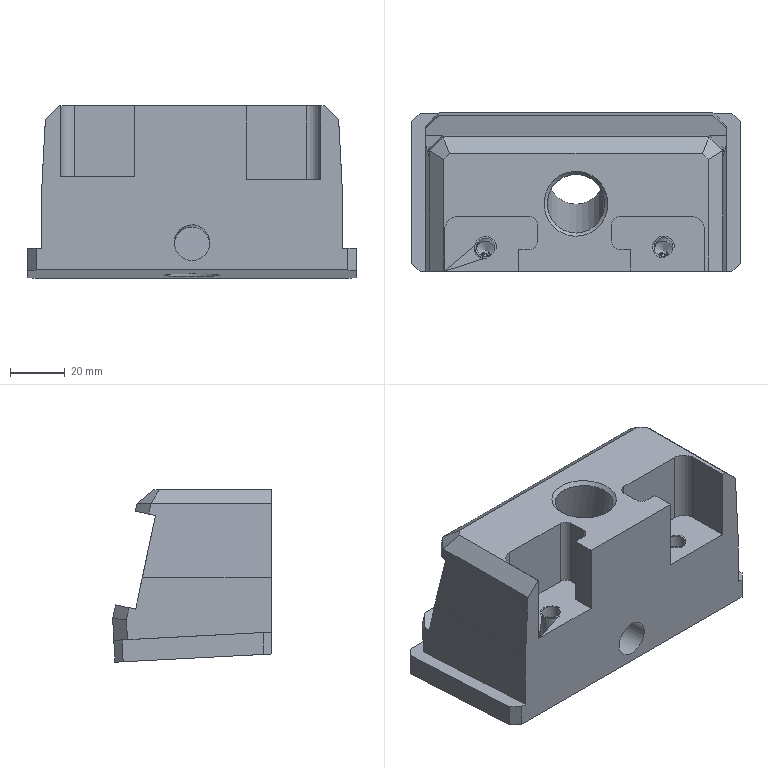Part | STEP file | P011002S001-000 | 1 solid | 195 faces | box 120 x 58 x 62.996 mm | volume 277812 mm3 | plane 122 | other 28 | cone 24 | cylinder 20 | spline 1 | commonest cylinder face diameters 6 x4 4.167 x2 4.983 x2 5 x2 6.8 x2 7.973 x2